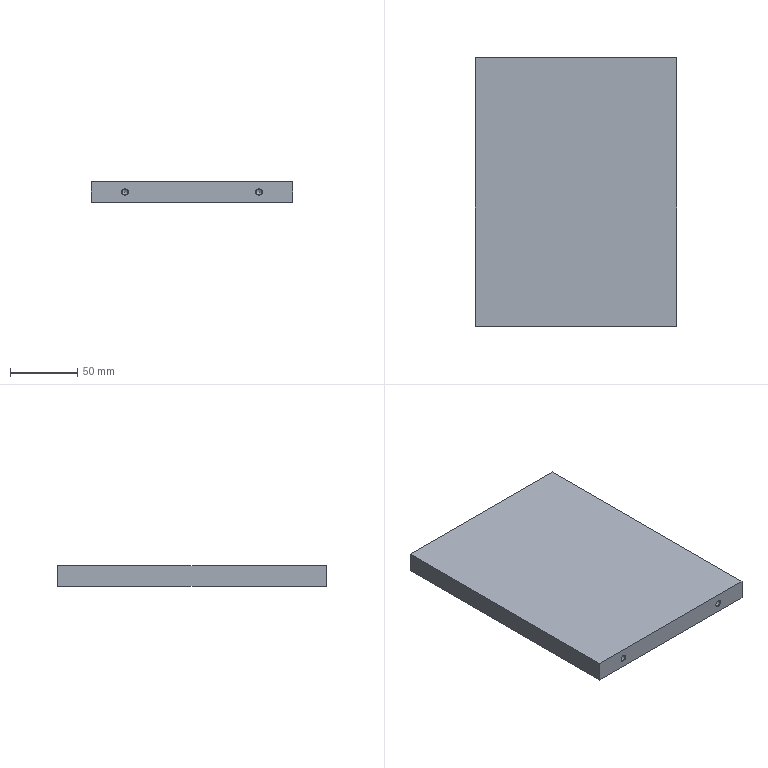Part | NX | features DATUM_CSYS 4, SIMPLE HOLE 4, SYMBOLIC_THREAD 4, SKETCH 3, EXTRACT_FACE 2, HOLE PACKAGE 2, EXTRUDE 1, Instance Feature 1, Mirror Feature 1 | 1 solid | 18 faces | box 150 x 200 x 15 mm | volume 448864 mm3 | cone 8 | plane 6 | cylinder 4 | commonest cylinder face diameters 4.2 x4
STEP:
#1=CARTESIAN_POINT('',(-75.,100.,0.));
#2=VERTEX_POINT('',#1);
#3=CARTESIAN_POINT('',(-75.,-100.,0.));
#4=VERTEX_POINT('',#3);
#5=CARTESIAN_POINT('',(-75.,100.,0.));
#6=DIRECTION('',(0.,-1.,0.));
#7=VECTOR('',#6,1000.);
#8=LINE('',#5,#7);
#9=EDGE_CURVE('',#2,#4,#8,.T.);
#10=ORIENTED_EDGE('',*,*,#9,.T.);
#11=CARTESIAN_POINT('',(-75.,-100.,15.));
#12=VERTEX_POINT('',#11);
#13=CARTESIAN_POINT('',(-75.,-100.,15.));
#14=DIRECTION('',(0.,0.,-1.));
#15=VECTOR('',#14,1000.);
#16=LINE('',#13,#15);
#17=EDGE_CURVE('',#12,#4,#16,.T.);
#18=ORIENTED_EDGE('',*,*,#17,.F.);
#19=CARTESIAN_POINT('',(-75.,100.,15.));
#20=VERTEX_POINT('',#19);
#21=CARTESIAN_POINT('',(-75.,100.,15.));
#22=DIRECTION('',(0.,-1.,0.));
#23=VECTOR('',#22,1000.);
#24=LINE('',#21,#23);
#25=EDGE_CURVE('',#20,#12,#24,.T.);
#26=ORIENTED_EDGE('',*,*,#25,.F.);
#27=CARTESIAN_POINT('',(-75.,100.,15.));
#28=DIRECTION('',(0.,0.,-1.));
#29=VECTOR('',#28,1000.);
#30=LINE('',#27,#29);
#31=EDGE_CURVE('',#20,#2,#30,.T.);
#32=ORIENTED_EDGE('',*,*,#31,.T.);
#33=EDGE_LOOP('',(#10,#18,#26,#32));
#34=FACE_BOUND('',#33,.T.);
#35=CARTESIAN_POINT('',(-75.,100.,15.));
#36=DIRECTION('',(1.,0.,0.));
#37=DIRECTION('',(0.,1.,0.));
#38=AXIS2_PLACEMENT_3D('',#35,#36,#37);
#39=PLANE('',#38);
#40=ADVANCED_FACE('',(#34),#39,.F.);
#41=CARTESIAN_POINT('',(50.,-100.,10.));
#42=VERTEX_POINT('',#41);
#43=CARTESIAN_POINT('',(50.,-100.,7.5));
#44=DIRECTION('',(0.,1.,0.));
#45=DIRECTION('',(0.,0.,1.));
#46=AXIS2_PLACEMENT_3D('',#43,#44,#45);
#47=CIRCLE('',#46,2.5);
#48=EDGE_CURVE('',#42,#42,#47,.T.);
#49=ORIENTED_EDGE('',*,*,#48,.T.);
#50=EDGE_LOOP('',(#49));
#51=FACE_BOUND('',#50,.T.);
#52=CARTESIAN_POINT('',(-50.,-100.,10.));
#53=VERTEX_POINT('',#52);
#54=CARTESIAN_POINT('',(-50.,-100.,7.5));
#55=DIRECTION('',(0.,1.,0.));
#56=DIRECTION('',(0.,0.,1.));
#57=AXIS2_PLACEMENT_3D('',#54,#55,#56);
#58=CIRCLE('',#57,2.5);
#59=EDGE_CURVE('',#53,#53,#58,.T.);
#60=ORIENTED_EDGE('',*,*,#59,.T.);
#61=EDGE_LOOP('',(#60));
#62=FACE_BOUND('',#61,.T.);
#63=CARTESIAN_POINT('',(75.,-100.,0.));
#64=VERTEX_POINT('',#63);
#65=CARTESIAN_POINT('',(-75.,-100.,0.));
#66=DIRECTION('',(1.,0.,0.));
#67=VECTOR('',#66,1000.);
#68=LINE('',#65,#67);
#69=EDGE_CURVE('',#4,#64,#68,.T.);
#70=ORIENTED_EDGE('',*,*,#69,.T.);
#71=CARTESIAN_POINT('',(75.,-100.,15.));
#72=VERTEX_POINT('',#71);
#73=CARTESIAN_POINT('',(75.,-100.,15.));
#74=DIRECTION('',(0.,0.,-1.));
#75=VECTOR('',#74,1000.);
#76=LINE('',#73,#75);
#77=EDGE_CURVE('',#72,#64,#76,.T.);
#78=ORIENTED_EDGE('',*,*,#77,.F.);
#79=CARTESIAN_POINT('',(-75.,-100.,15.));
#80=DIRECTION('',(1.,0.,0.));
#81=VECTOR('',#80,1000.);
#82=LINE('',#79,#81);
#83=EDGE_CURVE('',#12,#72,#82,.T.);
#84=ORIENTED_EDGE('',*,*,#83,.F.);
#85=ORIENTED_EDGE('',*,*,#17,.T.);
#86=EDGE_LOOP('',(#70,#78,#84,#85));
#87=FACE_BOUND('',#86,.T.);
#88=CARTESIAN_POINT('',(-75.,-100.,15.));
#89=DIRECTION('',(0.,1.,0.));
#90=DIRECTION('',(0.,0.,1.));
#91=AXIS2_PLACEMENT_3D('',#88,#89,#90);
#92=PLANE('',#91);
#93=ADVANCED_FACE('',(#51,#62,#87),#92,.F.);
#94=CARTESIAN_POINT('',(75.,100.,0.));
#95=VERTEX_POINT('',#94);
#96=CARTESIAN_POINT('',(75.,-100.,0.));
#97=DIRECTION('',(0.,1.,0.));
#98=VECTOR('',#97,1000.);
#99=LINE('',#96,#98);
#100=EDGE_CURVE('',#64,#95,#99,.T.);
#101=ORIENTED_EDGE('',*,*,#100,.T.);
#102=CARTESIAN_POINT('',(75.,100.,15.));
#103=VERTEX_POINT('',#102);
#104=CARTESIAN_POINT('',(75.,100.,15.));
#105=DIRECTION('',(0.,0.,-1.));
#106=VECTOR('',#105,1000.);
#107=LINE('',#104,#106);
#108=EDGE_CURVE('',#103,#95,#107,.T.);
#109=ORIENTED_EDGE('',*,*,#108,.F.);
#110=CARTESIAN_POINT('',(75.,-100.,15.));
#111=DIRECTION('',(0.,1.,0.));
#112=VECTOR('',#111,1000.);
#113=LINE('',#110,#112);
#114=EDGE_CURVE('',#72,#103,#113,.T.);
#115=ORIENTED_EDGE('',*,*,#114,.F.);
#116=ORIENTED_EDGE('',*,*,#77,.T.);
#117=EDGE_LOOP('',(#101,#109,#115,#116));
#118=FACE_BOUND('',#117,.T.);
#119=CARTESIAN_POINT('',(75.,-100.,15.));
#120=DIRECTION('',(-1.,0.,0.));
#121=DIRECTION('',(0.,-1.,0.));
#122=AXIS2_PLACEMENT_3D('',#119,#120,#121);
#123=PLANE('',#122);
#124=ADVANCED_FACE('',(#118),#123,.F.);
#125=CARTESIAN_POINT('',(50.,100.,5.));
#126=VERTEX_POINT('',#125);
#127=CARTESIAN_POINT('',(50.,100.,7.5));
#128=DIRECTION('',(0.,-1.,0.));
#129=DIRECTION('',(0.,0.,-1.));
#130=AXIS2_PLACEMENT_3D('',#127,#128,#129);
#131=CIRCLE('',#130,2.5);
#132=EDGE_CURVE('',#126,#126,#131,.T.);
#133=ORIENTED_EDGE('',*,*,#132,.T.);
#134=EDGE_LOOP('',(#133));
#135=FACE_BOUND('',#134,.T.);
#136=CARTESIAN_POINT('',(-50.,100.,5.));
#137=VERTEX_POINT('',#136);
#138=CARTESIAN_POINT('',(-50.,100.,7.5));
#139=DIRECTION('',(0.,-1.,0.));
#140=DIRECTION('',(0.,0.,-1.));
#141=AXIS2_PLACEMENT_3D('',#138,#139,#140);
#142=CIRCLE('',#141,2.5);
#143=EDGE_CURVE('',#137,#137,#142,.T.);
#144=ORIENTED_EDGE('',*,*,#143,.T.);
#145=EDGE_LOOP('',(#144));
#146=FACE_BOUND('',#145,.T.);
#147=CARTESIAN_POINT('',(75.,100.,0.));
#148=DIRECTION('',(-1.,0.,0.));
#149=VECTOR('',#148,1000.);
#150=LINE('',#147,#149);
#151=EDGE_CURVE('',#95,#2,#150,.T.);
#152=ORIENTED_EDGE('',*,*,#151,.T.);
#153=ORIENTED_EDGE('',*,*,#31,.F.);
#154=CARTESIAN_POINT('',(75.,100.,15.));
#155=DIRECTION('',(-1.,0.,0.));
#156=VECTOR('',#155,1000.);
#157=LINE('',#154,#156);
#158=EDGE_CURVE('',#103,#20,#157,.T.);
#159=ORIENTED_EDGE('',*,*,#158,.F.);
#160=ORIENTED_EDGE('',*,*,#108,.T.);
#161=EDGE_LOOP('',(#152,#153,#159,#160));
#162=FACE_BOUND('',#161,.T.);
#163=CARTESIAN_POINT('',(75.,100.,15.));
#164=DIRECTION('',(0.,-1.,0.));
#165=DIRECTION('',(0.,0.,-1.));
#166=AXIS2_PLACEMENT_3D('',#163,#164,#165);
#167=PLANE('',#166);
#168=ADVANCED_FACE('',(#135,#146,#162),#167,.F.);
#169=ORIENTED_EDGE('',*,*,#25,.T.);
#170=ORIENTED_EDGE('',*,*,#83,.T.);
#171=ORIENTED_EDGE('',*,*,#114,.T.);
#172=ORIENTED_EDGE('',*,*,#158,.T.);
#173=EDGE_LOOP('',(#169,#170,#171,#172));
#174=FACE_BOUND('',#173,.T.);
#175=CARTESIAN_POINT('',(0.,0.,15.));
#176=DIRECTION('',(0.,0.,1.));
#177=DIRECTION('',(1.,0.,0.));
#178=AXIS2_PLACEMENT_3D('',#175,#176,#177);
#179=PLANE('',#178);
#180=ADVANCED_FACE('',(#174),#179,.T.);
#181=ORIENTED_EDGE('',*,*,#9,.F.);
#182=ORIENTED_EDGE('',*,*,#151,.F.);
#183=ORIENTED_EDGE('',*,*,#100,.F.);
#184=ORIENTED_EDGE('',*,*,#69,.F.);
#185=EDGE_LOOP('',(#181,#182,#183,#184));
#186=FACE_BOUND('',#185,.T.);
#187=CARTESIAN_POINT('',(0.,0.,0.));
#188=DIRECTION('',(0.,0.,1.));
#189=DIRECTION('',(1.,0.,0.));
#190=AXIS2_PLACEMENT_3D('',#187,#188,#189);
#191=PLANE('',#190);
#192=ADVANCED_FACE('',(#186),#191,.F.);
#193=CARTESIAN_POINT('',(-50.,80.,5.4));
#194=VERTEX_POINT('',#193);
#195=CARTESIAN_POINT('',(-50.,80.,7.5));
#196=DIRECTION('',(0.,-1.,0.));
#197=DIRECTION('',(0.,0.,-1.));
#198=AXIS2_PLACEMENT_3D('',#195,#196,#197);
#199=CIRCLE('',#198,2.1);
#200=EDGE_CURVE('',#194,#194,#199,.F.);
#201=ORIENTED_EDGE('',*,*,#200,.T.);
#202=EDGE_LOOP('',(#201));
#203=FACE_BOUND('',#202,.T.);
#204=CARTESIAN_POINT('',(-50.,78.738,7.5));
#205=VERTEX_POINT('',#204);
#206=VERTEX_LOOP('',#205);
#207=FACE_BOUND('',#206,.T.);
#208=CARTESIAN_POINT('',(-50.,80.,7.5));
#209=DIRECTION('',(0.,1.,0.));
#210=DIRECTION('',(0.,0.,1.));
#211=AXIS2_PLACEMENT_3D('',#208,#209,#210);
#212=CONICAL_SURFACE('',#211,2.1,1.03);
#213=ADVANCED_FACE('',(#203,#207),#212,.F.);
#214=CARTESIAN_POINT('',(-50.,99.6,5.4));
#215=VERTEX_POINT('',#214);
#216=CARTESIAN_POINT('',(-50.,99.6,7.5));
#217=DIRECTION('',(0.,-1.,0.));
#218=DIRECTION('',(0.,0.,-1.));
#219=AXIS2_PLACEMENT_3D('',#216,#217,#218);
#220=CIRCLE('',#219,2.1);
#221=EDGE_CURVE('',#215,#215,#220,.F.);
#222=ORIENTED_EDGE('',*,*,#221,.T.);
#223=EDGE_LOOP('',(#222));
#224=FACE_BOUND('',#223,.T.);
#225=ORIENTED_EDGE('',*,*,#200,.F.);
#226=EDGE_LOOP('',(#225));
#227=FACE_BOUND('',#226,.T.);
#228=CARTESIAN_POINT('',(-50.,100.,7.5));
#229=DIRECTION('',(0.,-1.,0.));
#230=DIRECTION('',(0.,0.,-1.));
#231=AXIS2_PLACEMENT_3D('',#228,#229,#230);
#232=CYLINDRICAL_SURFACE('',#231,2.1);
#233=ADVANCED_FACE('',(#224,#227),#232,.F.);
#234=ORIENTED_EDGE('',*,*,#221,.F.);
#235=EDGE_LOOP('',(#234));
#236=FACE_BOUND('',#235,.T.);
#237=ORIENTED_EDGE('',*,*,#143,.F.);
#238=EDGE_LOOP('',(#237));
#239=FACE_BOUND('',#238,.T.);
#240=CARTESIAN_POINT('',(-50.,100.,7.5));
#241=DIRECTION('',(0.,1.,0.));
#242=DIRECTION('',(0.,0.,1.));
#243=AXIS2_PLACEMENT_3D('',#240,#241,#242);
#244=CONICAL_SURFACE('',#243,2.5,0.7854);
#245=ADVANCED_FACE('',(#236,#239),#244,.F.);
#246=CARTESIAN_POINT('',(50.,80.,5.4));
#247=VERTEX_POINT('',#246);
#248=CARTESIAN_POINT('',(50.,80.,7.5));
#249=DIRECTION('',(0.,-1.,0.));
#250=DIRECTION('',(0.,0.,-1.));
#251=AXIS2_PLACEMENT_3D('',#248,#249,#250);
#252=CIRCLE('',#251,2.1);
#253=EDGE_CURVE('',#247,#247,#252,.F.);
#254=ORIENTED_EDGE('',*,*,#253,.T.);
#255=EDGE_LOOP('',(#254));
#256=FACE_BOUND('',#255,.T.);
#257=CARTESIAN_POINT('',(50.,78.738,7.5));
#258=VERTEX_POINT('',#257);
#259=VERTEX_LOOP('',#258);
#260=FACE_BOUND('',#259,.T.);
#261=CARTESIAN_POINT('',(50.,80.,7.5));
#262=DIRECTION('',(0.,1.,0.));
#263=DIRECTION('',(0.,0.,1.));
#264=AXIS2_PLACEMENT_3D('',#261,#262,#263);
#265=CONICAL_SURFACE('',#264,2.1,1.03);
#266=ADVANCED_FACE('',(#256,#260),#265,.F.);
#267=CARTESIAN_POINT('',(50.,99.6,5.4));
#268=VERTEX_POINT('',#267);
#269=CARTESIAN_POINT('',(50.,99.6,7.5));
#270=DIRECTION('',(0.,-1.,0.));
#271=DIRECTION('',(0.,0.,-1.));
#272=AXIS2_PLACEMENT_3D('',#269,#270,#271);
#273=CIRCLE('',#272,2.1);
#274=EDGE_CURVE('',#268,#268,#273,.F.);
#275=ORIENTED_EDGE('',*,*,#274,.T.);
#276=EDGE_LOOP('',(#275));
#277=FACE_BOUND('',#276,.T.);
#278=ORIENTED_EDGE('',*,*,#253,.F.);
#279=EDGE_LOOP('',(#278));
#280=FACE_BOUND('',#279,.T.);
#281=CARTESIAN_POINT('',(50.,100.,7.5));
#282=DIRECTION('',(0.,-1.,0.));
#283=DIRECTION('',(0.,0.,-1.));
#284=AXIS2_PLACEMENT_3D('',#281,#282,#283);
#285=CYLINDRICAL_SURFACE('',#284,2.1);
#286=ADVANCED_FACE('',(#277,#280),#285,.F.);
#287=ORIENTED_EDGE('',*,*,#274,.F.);
#288=EDGE_LOOP('',(#287));
#289=FACE_BOUND('',#288,.T.);
#290=ORIENTED_EDGE('',*,*,#132,.F.);
#291=EDGE_LOOP('',(#290));
#292=FACE_BOUND('',#291,.T.);
#293=CARTESIAN_POINT('',(50.,100.,7.5));
#294=DIRECTION('',(0.,1.,0.));
#295=DIRECTION('',(0.,0.,1.));
#296=AXIS2_PLACEMENT_3D('',#293,#294,#295);
#297=CONICAL_SURFACE('',#296,2.5,0.7854);
#298=ADVANCED_FACE('',(#289,#292),#297,.F.);
#299=CARTESIAN_POINT('',(-50.,-80.,9.6));
#300=VERTEX_POINT('',#299);
#301=CARTESIAN_POINT('',(-50.,-80.,7.5));
#302=DIRECTION('',(0.,1.,0.));
#303=DIRECTION('',(0.,0.,1.));
#304=AXIS2_PLACEMENT_3D('',#301,#302,#303);
#305=CIRCLE('',#304,2.1);
#306=EDGE_CURVE('',#300,#300,#305,.T.);
#307=ORIENTED_EDGE('',*,*,#306,.F.);
#308=EDGE_LOOP('',(#307));
#309=FACE_BOUND('',#308,.T.);
#310=CARTESIAN_POINT('',(-50.,-78.738,7.5));
#311=VERTEX_POINT('',#310);
#312=VERTEX_LOOP('',#311);
#313=FACE_BOUND('',#312,.T.);
#314=CARTESIAN_POINT('',(-50.,-80.,7.5));
#315=DIRECTION('',(0.,-1.,0.));
#316=DIRECTION('',(0.,0.,-1.));
#317=AXIS2_PLACEMENT_3D('',#314,#315,#316);
#318=CONICAL_SURFACE('',#317,2.1,1.03);
#319=ADVANCED_FACE('',(#309,#313),#318,.F.);
#320=CARTESIAN_POINT('',(-50.,-99.6,9.6));
#321=VERTEX_POINT('',#320);
#322=CARTESIAN_POINT('',(-50.,-99.6,7.5));
#323=DIRECTION('',(0.,1.,0.));
#324=DIRECTION('',(0.,0.,1.));
#325=AXIS2_PLACEMENT_3D('',#322,#323,#324);
#326=CIRCLE('',#325,2.1);
#327=EDGE_CURVE('',#321,#321,#326,.T.);
#328=ORIENTED_EDGE('',*,*,#327,.F.);
#329=EDGE_LOOP('',(#328));
#330=FACE_BOUND('',#329,.T.);
#331=ORIENTED_EDGE('',*,*,#306,.T.);
#332=EDGE_LOOP('',(#331));
#333=FACE_BOUND('',#332,.T.);
#334=CARTESIAN_POINT('',(-50.,-100.,7.5));
#335=DIRECTION('',(0.,1.,0.));
#336=DIRECTION('',(0.,0.,1.));
#337=AXIS2_PLACEMENT_3D('',#334,#335,#336);
#338=CYLINDRICAL_SURFACE('',#337,2.1);
#339=ADVANCED_FACE('',(#330,#333),#338,.F.);
#340=ORIENTED_EDGE('',*,*,#327,.T.);
#341=EDGE_LOOP('',(#340));
#342=FACE_BOUND('',#341,.T.);
#343=ORIENTED_EDGE('',*,*,#59,.F.);
#344=EDGE_LOOP('',(#343));
#345=FACE_BOUND('',#344,.T.);
#346=CARTESIAN_POINT('',(-50.,-100.,7.5));
#347=DIRECTION('',(0.,-1.,0.));
#348=DIRECTION('',(0.,0.,-1.));
#349=AXIS2_PLACEMENT_3D('',#346,#347,#348);
#350=CONICAL_SURFACE('',#349,2.5,0.7854);
#351=ADVANCED_FACE('',(#342,#345),#350,.F.);
#352=CARTESIAN_POINT('',(50.,-80.,9.6));
#353=VERTEX_POINT('',#352);
#354=CARTESIAN_POINT('',(50.,-80.,7.5));
#355=DIRECTION('',(0.,1.,0.));
#356=DIRECTION('',(0.,0.,1.));
#357=AXIS2_PLACEMENT_3D('',#354,#355,#356);
#358=CIRCLE('',#357,2.1);
#359=EDGE_CURVE('',#353,#353,#358,.T.);
#360=ORIENTED_EDGE('',*,*,#359,.F.);
#361=EDGE_LOOP('',(#360));
#362=FACE_BOUND('',#361,.T.);
#363=CARTESIAN_POINT('',(50.,-78.738,7.5));
#364=VERTEX_POINT('',#363);
#365=VERTEX_LOOP('',#364);
#366=FACE_BOUND('',#365,.T.);
#367=CARTESIAN_POINT('',(50.,-80.,7.5));
#368=DIRECTION('',(0.,-1.,0.));
#369=DIRECTION('',(0.,0.,-1.));
#370=AXIS2_PLACEMENT_3D('',#367,#368,#369);
#371=CONICAL_SURFACE('',#370,2.1,1.03);
#372=ADVANCED_FACE('',(#362,#366),#371,.F.);
#373=CARTESIAN_POINT('',(50.,-99.6,9.6));
#374=VERTEX_POINT('',#373);
#375=CARTESIAN_POINT('',(50.,-99.6,7.5));
#376=DIRECTION('',(0.,1.,0.));
#377=DIRECTION('',(0.,0.,1.));
#378=AXIS2_PLACEMENT_3D('',#375,#376,#377);
#379=CIRCLE('',#378,2.1);
#380=EDGE_CURVE('',#374,#374,#379,.T.);
#381=ORIENTED_EDGE('',*,*,#380,.F.);
#382=EDGE_LOOP('',(#381));
#383=FACE_BOUND('',#382,.T.);
#384=ORIENTED_EDGE('',*,*,#359,.T.);
#385=EDGE_LOOP('',(#384));
#386=FACE_BOUND('',#385,.T.);
#387=CARTESIAN_POINT('',(50.,-100.,7.5));
#388=DIRECTION('',(0.,1.,0.));
#389=DIRECTION('',(0.,0.,1.));
#390=AXIS2_PLACEMENT_3D('',#387,#388,#389);
#391=CYLINDRICAL_SURFACE('',#390,2.1);
#392=ADVANCED_FACE('',(#383,#386),#391,.F.);
#393=ORIENTED_EDGE('',*,*,#380,.T.);
#394=EDGE_LOOP('',(#393));
#395=FACE_BOUND('',#394,.T.);
#396=ORIENTED_EDGE('',*,*,#48,.F.);
#397=EDGE_LOOP('',(#396));
#398=FACE_BOUND('',#397,.T.);
#399=CARTESIAN_POINT('',(50.,-100.,7.5));
#400=DIRECTION('',(0.,-1.,0.));
#401=DIRECTION('',(0.,0.,-1.));
#402=AXIS2_PLACEMENT_3D('',#399,#400,#401);
#403=CONICAL_SURFACE('',#402,2.5,0.7854);
#404=ADVANCED_FACE('',(#395,#398),#403,.F.);
#405=CLOSED_SHELL('',(#40,#93,#124,#168,#180,#192,#213,#233,#245,#266,#286,#298,#319,#339,#351,#372,#392,#404));
#406=MANIFOLD_SOLID_BREP('',#405);
#407=(LENGTH_UNIT()NAMED_UNIT(*)SI_UNIT(.MILLI.,.METRE.));
#408=UNCERTAINTY_MEASURE_WITH_UNIT(LENGTH_MEASURE(0.00001),#407,'','');
#409=(NAMED_UNIT(*)PLANE_ANGLE_UNIT()SI_UNIT($,.RADIAN.));
#410=(NAMED_UNIT(*)SI_UNIT($,.STERADIAN.)SOLID_ANGLE_UNIT());
#411=(GEOMETRIC_REPRESENTATION_CONTEXT(3)GLOBAL_UNCERTAINTY_ASSIGNED_CONTEXT((#408))GLOBAL_UNIT_ASSIGNED_CONTEXT((#407,#409,#410))REPRESENTATION_CONTEXT('',''));
#412=ADVANCED_BREP_SHAPE_REPRESENTATION('',(#406),#411);